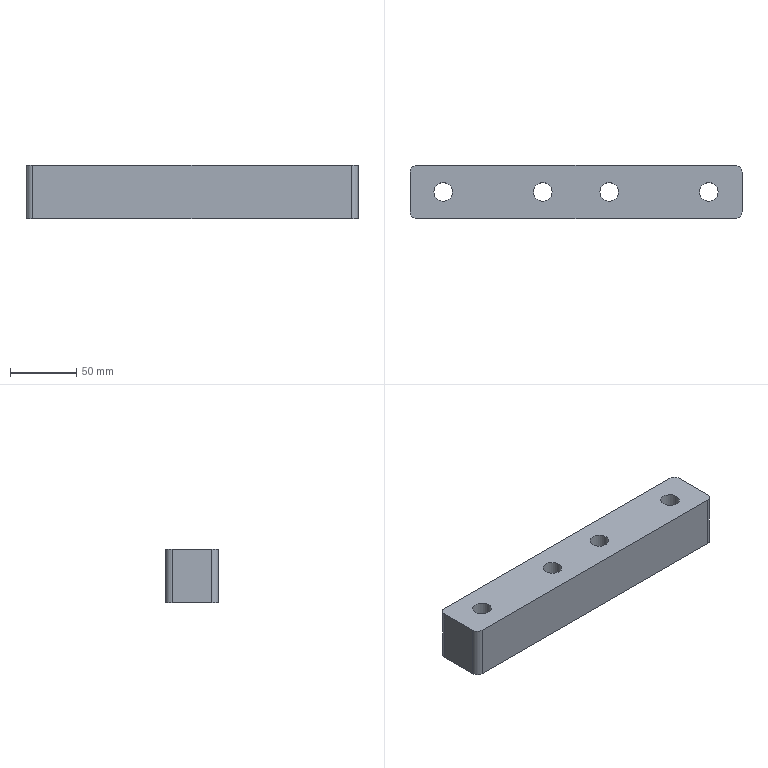Part | NX | features MAIN_BODY 2 | 1 solid | 14 faces | box 250 x 40 x 40 mm | volume 374512 mm3 | cylinder 8 | plane 6 | commonest cylinder face diameters 10 x4 14 x4
STEP:
#1=CARTESIAN_POINT('',(245.,825.,-195.));
#2=VERTEX_POINT('',#1);
#3=CARTESIAN_POINT('',(245.,795.,-195.));
#4=VERTEX_POINT('',#3);
#5=CARTESIAN_POINT('',(245.,830.,-195.));
#6=DIRECTION('',(0.,-1.,0.));
#7=VECTOR('',#6,1000.);
#8=LINE('',#5,#7);
#9=EDGE_CURVE('',#2,#4,#8,.T.);
#10=ORIENTED_EDGE('',*,*,#9,.F.);
#11=CARTESIAN_POINT('',(245.,825.,-235.));
#12=VERTEX_POINT('',#11);
#13=CARTESIAN_POINT('',(245.,825.,-235.));
#14=DIRECTION('',(0.,0.,1.));
#15=VECTOR('',#14,1000.);
#16=LINE('',#13,#15);
#17=EDGE_CURVE('',#2,#12,#16,.F.);
#18=ORIENTED_EDGE('',*,*,#17,.T.);
#19=CARTESIAN_POINT('',(245.,795.,-235.));
#20=VERTEX_POINT('',#19);
#21=CARTESIAN_POINT('',(245.,830.,-235.));
#22=DIRECTION('',(0.,-1.,0.));
#23=VECTOR('',#22,1000.);
#24=LINE('',#21,#23);
#25=EDGE_CURVE('',#12,#20,#24,.T.);
#26=ORIENTED_EDGE('',*,*,#25,.T.);
#27=CARTESIAN_POINT('',(245.,795.,-235.));
#28=DIRECTION('',(0.,0.,1.));
#29=VECTOR('',#28,1000.);
#30=LINE('',#27,#29);
#31=EDGE_CURVE('',#20,#4,#30,.T.);
#32=ORIENTED_EDGE('',*,*,#31,.T.);
#33=EDGE_LOOP('',(#10,#18,#26,#32));
#34=FACE_BOUND('',#33,.T.);
#35=CARTESIAN_POINT('',(245.,830.,-235.));
#36=DIRECTION('',(-1.,0.,0.));
#37=DIRECTION('',(0.,1.,0.));
#38=AXIS2_PLACEMENT_3D('',#35,#36,#37);
#39=PLANE('',#38);
#40=ADVANCED_FACE('',(#34),#39,.T.);
#41=CARTESIAN_POINT('',(250.,790.,-195.));
#42=VERTEX_POINT('',#41);
#43=CARTESIAN_POINT('',(490.,790.,-195.));
#44=VERTEX_POINT('',#43);
#45=CARTESIAN_POINT('',(245.,790.,-195.));
#46=DIRECTION('',(1.,0.,0.));
#47=VECTOR('',#46,1000.);
#48=LINE('',#45,#47);
#49=EDGE_CURVE('',#42,#44,#48,.T.);
#50=ORIENTED_EDGE('',*,*,#49,.F.);
#51=CARTESIAN_POINT('',(250.,790.,-235.));
#52=VERTEX_POINT('',#51);
#53=CARTESIAN_POINT('',(250.,790.,-235.));
#54=DIRECTION('',(0.,0.,1.));
#55=VECTOR('',#54,1000.);
#56=LINE('',#53,#55);
#57=EDGE_CURVE('',#42,#52,#56,.F.);
#58=ORIENTED_EDGE('',*,*,#57,.T.);
#59=CARTESIAN_POINT('',(490.,790.,-235.));
#60=VERTEX_POINT('',#59);
#61=CARTESIAN_POINT('',(245.,790.,-235.));
#62=DIRECTION('',(1.,0.,0.));
#63=VECTOR('',#62,1000.);
#64=LINE('',#61,#63);
#65=EDGE_CURVE('',#52,#60,#64,.T.);
#66=ORIENTED_EDGE('',*,*,#65,.T.);
#67=CARTESIAN_POINT('',(490.,790.,-235.));
#68=DIRECTION('',(0.,0.,1.));
#69=VECTOR('',#68,1000.);
#70=LINE('',#67,#69);
#71=EDGE_CURVE('',#60,#44,#70,.T.);
#72=ORIENTED_EDGE('',*,*,#71,.T.);
#73=EDGE_LOOP('',(#50,#58,#66,#72));
#74=FACE_BOUND('',#73,.T.);
#75=CARTESIAN_POINT('',(245.,790.,-235.));
#76=DIRECTION('',(0.,-1.,0.));
#77=DIRECTION('',(-1.,0.,0.));
#78=AXIS2_PLACEMENT_3D('',#75,#76,#77);
#79=PLANE('',#78);
#80=ADVANCED_FACE('',(#74),#79,.T.);
#81=CARTESIAN_POINT('',(490.,830.,-235.));
#82=VERTEX_POINT('',#81);
#83=CARTESIAN_POINT('',(250.,830.,-235.));
#84=VERTEX_POINT('',#83);
#85=CARTESIAN_POINT('',(370.,830.,-235.));
#86=DIRECTION('',(-1.,0.,0.));
#87=VECTOR('',#86,1000.);
#88=LINE('',#85,#87);
#89=EDGE_CURVE('',#82,#84,#88,.T.);
#90=ORIENTED_EDGE('',*,*,#89,.T.);
#91=CARTESIAN_POINT('',(250.,830.,-195.));
#92=VERTEX_POINT('',#91);
#93=CARTESIAN_POINT('',(250.,830.,-235.));
#94=DIRECTION('',(0.,0.,1.));
#95=VECTOR('',#94,1000.);
#96=LINE('',#93,#95);
#97=EDGE_CURVE('',#84,#92,#96,.T.);
#98=ORIENTED_EDGE('',*,*,#97,.T.);
#99=CARTESIAN_POINT('',(490.,830.,-195.));
#100=VERTEX_POINT('',#99);
#101=CARTESIAN_POINT('',(370.,830.,-195.));
#102=DIRECTION('',(-1.,0.,0.));
#103=VECTOR('',#102,1000.);
#104=LINE('',#101,#103);
#105=EDGE_CURVE('',#100,#92,#104,.T.);
#106=ORIENTED_EDGE('',*,*,#105,.F.);
#107=CARTESIAN_POINT('',(490.,830.,-235.));
#108=DIRECTION('',(0.,0.,1.));
#109=VECTOR('',#108,1000.);
#110=LINE('',#107,#109);
#111=EDGE_CURVE('',#100,#82,#110,.F.);
#112=ORIENTED_EDGE('',*,*,#111,.T.);
#113=EDGE_LOOP('',(#90,#98,#106,#112));
#114=FACE_BOUND('',#113,.T.);
#115=CARTESIAN_POINT('',(370.,830.,-235.));
#116=DIRECTION('',(0.,1.,0.));
#117=DIRECTION('',(0.,0.,-1.));
#118=AXIS2_PLACEMENT_3D('',#115,#116,#117);
#119=PLANE('',#118);
#120=ADVANCED_FACE('',(#114),#119,.T.);
#121=CARTESIAN_POINT('',(352.,810.,-235.));
#122=VERTEX_POINT('',#121);
#123=CARTESIAN_POINT('',(345.,810.,-235.));
#124=DIRECTION('',(0.,0.,1.));
#125=DIRECTION('',(1.,0.,0.));
#126=AXIS2_PLACEMENT_3D('',#123,#124,#125);
#127=CIRCLE('',#126,7.);
#128=EDGE_CURVE('',#122,#122,#127,.T.);
#129=ORIENTED_EDGE('',*,*,#128,.T.);
#130=EDGE_LOOP('',(#129));
#131=FACE_BOUND('',#130,.T.);
#132=CARTESIAN_POINT('',(277.,810.,-235.));
#133=VERTEX_POINT('',#132);
#134=CARTESIAN_POINT('',(270.,810.,-235.));
#135=DIRECTION('',(0.,0.,1.));
#136=DIRECTION('',(1.,0.,0.));
#137=AXIS2_PLACEMENT_3D('',#134,#135,#136);
#138=CIRCLE('',#137,7.);
#139=EDGE_CURVE('',#133,#133,#138,.T.);
#140=ORIENTED_EDGE('',*,*,#139,.T.);
#141=EDGE_LOOP('',(#140));
#142=FACE_BOUND('',#141,.T.);
#143=ORIENTED_EDGE('',*,*,#25,.F.);
#144=CARTESIAN_POINT('',(250.,825.,-235.));
#145=DIRECTION('',(0.,0.,1.));
#146=DIRECTION('',(1.,0.,0.));
#147=AXIS2_PLACEMENT_3D('',#144,#145,#146);
#148=CIRCLE('',#147,5.);
#149=EDGE_CURVE('',#12,#84,#148,.F.);
#150=ORIENTED_EDGE('',*,*,#149,.T.);
#151=ORIENTED_EDGE('',*,*,#89,.F.);
#152=CARTESIAN_POINT('',(495.,825.,-235.));
#153=VERTEX_POINT('',#152);
#154=CARTESIAN_POINT('',(490.,825.,-235.));
#155=DIRECTION('',(0.,0.,1.));
#156=DIRECTION('',(1.,0.,0.));
#157=AXIS2_PLACEMENT_3D('',#154,#155,#156);
#158=CIRCLE('',#157,5.);
#159=EDGE_CURVE('',#82,#153,#158,.F.);
#160=ORIENTED_EDGE('',*,*,#159,.T.);
#161=CARTESIAN_POINT('',(495.,795.,-235.));
#162=VERTEX_POINT('',#161);
#163=CARTESIAN_POINT('',(495.,830.,-235.));
#164=DIRECTION('',(0.,-1.,0.));
#165=VECTOR('',#164,1000.);
#166=LINE('',#163,#165);
#167=EDGE_CURVE('',#153,#162,#166,.T.);
#168=ORIENTED_EDGE('',*,*,#167,.T.);
#169=CARTESIAN_POINT('',(490.,795.,-235.));
#170=DIRECTION('',(0.,0.,1.));
#171=DIRECTION('',(1.,0.,0.));
#172=AXIS2_PLACEMENT_3D('',#169,#170,#171);
#173=CIRCLE('',#172,5.);
#174=EDGE_CURVE('',#162,#60,#173,.F.);
#175=ORIENTED_EDGE('',*,*,#174,.T.);
#176=ORIENTED_EDGE('',*,*,#65,.F.);
#177=CARTESIAN_POINT('',(250.,795.,-235.));
#178=DIRECTION('',(0.,0.,1.));
#179=DIRECTION('',(1.,0.,0.));
#180=AXIS2_PLACEMENT_3D('',#177,#178,#179);
#181=CIRCLE('',#180,5.);
#182=EDGE_CURVE('',#52,#20,#181,.F.);
#183=ORIENTED_EDGE('',*,*,#182,.T.);
#184=EDGE_LOOP('',(#143,#150,#151,#160,#168,#175,#176,#183));
#185=FACE_BOUND('',#184,.T.);
#186=CARTESIAN_POINT('',(388.,810.,-235.));
#187=VERTEX_POINT('',#186);
#188=CARTESIAN_POINT('',(395.,810.,-235.));
#189=DIRECTION('',(0.,0.,-1.));
#190=DIRECTION('',(-1.,0.,0.));
#191=AXIS2_PLACEMENT_3D('',#188,#189,#190);
#192=CIRCLE('',#191,7.);
#193=EDGE_CURVE('',#187,#187,#192,.T.);
#194=ORIENTED_EDGE('',*,*,#193,.F.);
#195=EDGE_LOOP('',(#194));
#196=FACE_BOUND('',#195,.T.);
#197=CARTESIAN_POINT('',(463.,810.,-235.));
#198=VERTEX_POINT('',#197);
#199=CARTESIAN_POINT('',(470.,810.,-235.));
#200=DIRECTION('',(0.,0.,-1.));
#201=DIRECTION('',(-1.,0.,0.));
#202=AXIS2_PLACEMENT_3D('',#199,#200,#201);
#203=CIRCLE('',#202,7.);
#204=EDGE_CURVE('',#198,#198,#203,.T.);
#205=ORIENTED_EDGE('',*,*,#204,.F.);
#206=EDGE_LOOP('',(#205));
#207=FACE_BOUND('',#206,.T.);
#208=CARTESIAN_POINT('',(245.,790.,-235.));
#209=DIRECTION('',(0.,0.,1.));
#210=DIRECTION('',(1.,0.,0.));
#211=AXIS2_PLACEMENT_3D('',#208,#209,#210);
#212=PLANE('',#211);
#213=ADVANCED_FACE('',(#131,#142,#185,#196,#207),#212,.F.);
#214=CARTESIAN_POINT('',(352.,810.,-195.));
#215=VERTEX_POINT('',#214);
#216=CARTESIAN_POINT('',(345.,810.,-195.));
#217=DIRECTION('',(0.,0.,1.));
#218=DIRECTION('',(1.,0.,0.));
#219=AXIS2_PLACEMENT_3D('',#216,#217,#218);
#220=CIRCLE('',#219,7.);
#221=EDGE_CURVE('',#215,#215,#220,.T.);
#222=ORIENTED_EDGE('',*,*,#221,.F.);
#223=EDGE_LOOP('',(#222));
#224=FACE_BOUND('',#223,.T.);
#225=CARTESIAN_POINT('',(277.,810.,-195.));
#226=VERTEX_POINT('',#225);
#227=CARTESIAN_POINT('',(270.,810.,-195.));
#228=DIRECTION('',(0.,0.,1.));
#229=DIRECTION('',(1.,0.,0.));
#230=AXIS2_PLACEMENT_3D('',#227,#228,#229);
#231=CIRCLE('',#230,7.);
#232=EDGE_CURVE('',#226,#226,#231,.T.);
#233=ORIENTED_EDGE('',*,*,#232,.F.);
#234=EDGE_LOOP('',(#233));
#235=FACE_BOUND('',#234,.T.);
#236=ORIENTED_EDGE('',*,*,#105,.T.);
#237=CARTESIAN_POINT('',(250.,825.,-195.));
#238=DIRECTION('',(0.,0.,1.));
#239=DIRECTION('',(1.,0.,0.));
#240=AXIS2_PLACEMENT_3D('',#237,#238,#239);
#241=CIRCLE('',#240,5.);
#242=EDGE_CURVE('',#92,#2,#241,.T.);
#243=ORIENTED_EDGE('',*,*,#242,.T.);
#244=ORIENTED_EDGE('',*,*,#9,.T.);
#245=CARTESIAN_POINT('',(250.,795.,-195.));
#246=DIRECTION('',(0.,0.,1.));
#247=DIRECTION('',(1.,0.,0.));
#248=AXIS2_PLACEMENT_3D('',#245,#246,#247);
#249=CIRCLE('',#248,5.);
#250=EDGE_CURVE('',#4,#42,#249,.T.);
#251=ORIENTED_EDGE('',*,*,#250,.T.);
#252=ORIENTED_EDGE('',*,*,#49,.T.);
#253=CARTESIAN_POINT('',(495.,795.,-195.));
#254=VERTEX_POINT('',#253);
#255=CARTESIAN_POINT('',(490.,795.,-195.));
#256=DIRECTION('',(0.,0.,1.));
#257=DIRECTION('',(1.,0.,0.));
#258=AXIS2_PLACEMENT_3D('',#255,#256,#257);
#259=CIRCLE('',#258,5.);
#260=EDGE_CURVE('',#44,#254,#259,.T.);
#261=ORIENTED_EDGE('',*,*,#260,.T.);
#262=CARTESIAN_POINT('',(495.,825.,-195.));
#263=VERTEX_POINT('',#262);
#264=CARTESIAN_POINT('',(495.,830.,-195.));
#265=DIRECTION('',(0.,-1.,0.));
#266=VECTOR('',#265,1000.);
#267=LINE('',#264,#266);
#268=EDGE_CURVE('',#263,#254,#267,.T.);
#269=ORIENTED_EDGE('',*,*,#268,.F.);
#270=CARTESIAN_POINT('',(490.,825.,-195.));
#271=DIRECTION('',(0.,0.,1.));
#272=DIRECTION('',(1.,0.,0.));
#273=AXIS2_PLACEMENT_3D('',#270,#271,#272);
#274=CIRCLE('',#273,5.);
#275=EDGE_CURVE('',#263,#100,#274,.T.);
#276=ORIENTED_EDGE('',*,*,#275,.T.);
#277=EDGE_LOOP('',(#236,#243,#244,#251,#252,#261,#269,#276));
#278=FACE_BOUND('',#277,.T.);
#279=CARTESIAN_POINT('',(388.,810.,-195.));
#280=VERTEX_POINT('',#279);
#281=CARTESIAN_POINT('',(395.,810.,-195.));
#282=DIRECTION('',(0.,0.,-1.));
#283=DIRECTION('',(-1.,0.,0.));
#284=AXIS2_PLACEMENT_3D('',#281,#282,#283);
#285=CIRCLE('',#284,7.);
#286=EDGE_CURVE('',#280,#280,#285,.T.);
#287=ORIENTED_EDGE('',*,*,#286,.T.);
#288=EDGE_LOOP('',(#287));
#289=FACE_BOUND('',#288,.T.);
#290=CARTESIAN_POINT('',(463.,810.,-195.));
#291=VERTEX_POINT('',#290);
#292=CARTESIAN_POINT('',(470.,810.,-195.));
#293=DIRECTION('',(0.,0.,-1.));
#294=DIRECTION('',(-1.,0.,0.));
#295=AXIS2_PLACEMENT_3D('',#292,#293,#294);
#296=CIRCLE('',#295,7.);
#297=EDGE_CURVE('',#291,#291,#296,.T.);
#298=ORIENTED_EDGE('',*,*,#297,.T.);
#299=EDGE_LOOP('',(#298));
#300=FACE_BOUND('',#299,.T.);
#301=CARTESIAN_POINT('',(245.,790.,-195.));
#302=DIRECTION('',(0.,0.,1.));
#303=DIRECTION('',(1.,0.,0.));
#304=AXIS2_PLACEMENT_3D('',#301,#302,#303);
#305=PLANE('',#304);
#306=ADVANCED_FACE('',(#224,#235,#278,#289,#300),#305,.T.);
#307=ORIENTED_EDGE('',*,*,#232,.T.);
#308=EDGE_LOOP('',(#307));
#309=FACE_BOUND('',#308,.T.);
#310=ORIENTED_EDGE('',*,*,#139,.F.);
#311=EDGE_LOOP('',(#310));
#312=FACE_BOUND('',#311,.T.);
#313=CARTESIAN_POINT('',(270.,810.,-235.));
#314=DIRECTION('',(0.,0.,1.));
#315=DIRECTION('',(1.,0.,0.));
#316=AXIS2_PLACEMENT_3D('',#313,#314,#315);
#317=CYLINDRICAL_SURFACE('',#316,7.);
#318=ADVANCED_FACE('',(#309,#312),#317,.F.);
#319=ORIENTED_EDGE('',*,*,#221,.T.);
#320=EDGE_LOOP('',(#319));
#321=FACE_BOUND('',#320,.T.);
#322=ORIENTED_EDGE('',*,*,#128,.F.);
#323=EDGE_LOOP('',(#322));
#324=FACE_BOUND('',#323,.T.);
#325=CARTESIAN_POINT('',(345.,810.,-235.));
#326=DIRECTION('',(0.,0.,1.));
#327=DIRECTION('',(1.,0.,0.));
#328=AXIS2_PLACEMENT_3D('',#325,#326,#327);
#329=CYLINDRICAL_SURFACE('',#328,7.);
#330=ADVANCED_FACE('',(#321,#324),#329,.F.);
#331=ORIENTED_EDGE('',*,*,#167,.F.);
#332=CARTESIAN_POINT('',(495.,825.,-235.));
#333=DIRECTION('',(0.,0.,1.));
#334=VECTOR('',#333,1000.);
#335=LINE('',#332,#334);
#336=EDGE_CURVE('',#153,#263,#335,.T.);
#337=ORIENTED_EDGE('',*,*,#336,.T.);
#338=ORIENTED_EDGE('',*,*,#268,.T.);
#339=CARTESIAN_POINT('',(495.,795.,-235.));
#340=DIRECTION('',(0.,0.,1.));
#341=VECTOR('',#340,1000.);
#342=LINE('',#339,#341);
#343=EDGE_CURVE('',#254,#162,#342,.F.);
#344=ORIENTED_EDGE('',*,*,#343,.T.);
#345=EDGE_LOOP('',(#331,#337,#338,#344));
#346=FACE_BOUND('',#345,.T.);
#347=CARTESIAN_POINT('',(495.,830.,-235.));
#348=DIRECTION('',(1.,0.,0.));
#349=DIRECTION('',(0.,1.,0.));
#350=AXIS2_PLACEMENT_3D('',#347,#348,#349);
#351=PLANE('',#350);
#352=ADVANCED_FACE('',(#346),#351,.T.);
#353=ORIENTED_EDGE('',*,*,#297,.F.);
#354=EDGE_LOOP('',(#353));
#355=FACE_BOUND('',#354,.T.);
#356=ORIENTED_EDGE('',*,*,#204,.T.);
#357=EDGE_LOOP('',(#356));
#358=FACE_BOUND('',#357,.T.);
#359=CARTESIAN_POINT('',(470.,810.,-235.));
#360=DIRECTION('',(0.,0.,1.));
#361=DIRECTION('',(-1.,0.,0.));
#362=AXIS2_PLACEMENT_3D('',#359,#360,#361);
#363=CYLINDRICAL_SURFACE('',#362,7.);
#364=ADVANCED_FACE('',(#355,#358),#363,.F.);
#365=ORIENTED_EDGE('',*,*,#286,.F.);
#366=EDGE_LOOP('',(#365));
#367=FACE_BOUND('',#366,.T.);
#368=ORIENTED_EDGE('',*,*,#193,.T.);
#369=EDGE_LOOP('',(#368));
#370=FACE_BOUND('',#369,.T.);
#371=CARTESIAN_POINT('',(395.,810.,-235.));
#372=DIRECTION('',(0.,0.,1.));
#373=DIRECTION('',(-1.,0.,0.));
#374=AXIS2_PLACEMENT_3D('',#371,#372,#373);
#375=CYLINDRICAL_SURFACE('',#374,7.);
#376=ADVANCED_FACE('',(#367,#370),#375,.F.);
#377=ORIENTED_EDGE('',*,*,#149,.F.);
#378=ORIENTED_EDGE('',*,*,#17,.F.);
#379=ORIENTED_EDGE('',*,*,#242,.F.);
#380=ORIENTED_EDGE('',*,*,#97,.F.);
#381=EDGE_LOOP('',(#377,#378,#379,#380));
#382=FACE_BOUND('',#381,.T.);
#383=CARTESIAN_POINT('',(250.,825.,-235.));
#384=DIRECTION('',(0.,0.,1.));
#385=DIRECTION('',(1.,0.,0.));
#386=AXIS2_PLACEMENT_3D('',#383,#384,#385);
#387=CYLINDRICAL_SURFACE('',#386,5.);
#388=ADVANCED_FACE('',(#382),#387,.T.);
#389=ORIENTED_EDGE('',*,*,#182,.F.);
#390=ORIENTED_EDGE('',*,*,#57,.F.);
#391=ORIENTED_EDGE('',*,*,#250,.F.);
#392=ORIENTED_EDGE('',*,*,#31,.F.);
#393=EDGE_LOOP('',(#389,#390,#391,#392));
#394=FACE_BOUND('',#393,.T.);
#395=CARTESIAN_POINT('',(250.,795.,-235.));
#396=DIRECTION('',(0.,0.,1.));
#397=DIRECTION('',(1.,0.,0.));
#398=AXIS2_PLACEMENT_3D('',#395,#396,#397);
#399=CYLINDRICAL_SURFACE('',#398,5.);
#400=ADVANCED_FACE('',(#394),#399,.T.);
#401=ORIENTED_EDGE('',*,*,#159,.F.);
#402=ORIENTED_EDGE('',*,*,#111,.F.);
#403=ORIENTED_EDGE('',*,*,#275,.F.);
#404=ORIENTED_EDGE('',*,*,#336,.F.);
#405=EDGE_LOOP('',(#401,#402,#403,#404));
#406=FACE_BOUND('',#405,.T.);
#407=CARTESIAN_POINT('',(490.,825.,-235.));
#408=DIRECTION('',(0.,0.,1.));
#409=DIRECTION('',(1.,0.,0.));
#410=AXIS2_PLACEMENT_3D('',#407,#408,#409);
#411=CYLINDRICAL_SURFACE('',#410,5.);
#412=ADVANCED_FACE('',(#406),#411,.T.);
#413=ORIENTED_EDGE('',*,*,#174,.F.);
#414=ORIENTED_EDGE('',*,*,#343,.F.);
#415=ORIENTED_EDGE('',*,*,#260,.F.);
#416=ORIENTED_EDGE('',*,*,#71,.F.);
#417=EDGE_LOOP('',(#413,#414,#415,#416));
#418=FACE_BOUND('',#417,.T.);
#419=CARTESIAN_POINT('',(490.,795.,-235.));
#420=DIRECTION('',(0.,0.,1.));
#421=DIRECTION('',(1.,0.,0.));
#422=AXIS2_PLACEMENT_3D('',#419,#420,#421);
#423=CYLINDRICAL_SURFACE('',#422,5.);
#424=ADVANCED_FACE('',(#418),#423,.T.);
#425=CLOSED_SHELL('',(#40,#80,#120,#213,#306,#318,#330,#352,#364,#376,#388,#400,#412,#424));
#426=MANIFOLD_SOLID_BREP('',#425);
#427=(LENGTH_UNIT()NAMED_UNIT(*)SI_UNIT(.MILLI.,.METRE.));
#428=UNCERTAINTY_MEASURE_WITH_UNIT(LENGTH_MEASURE(0.00001),#427,'','');
#429=(NAMED_UNIT(*)PLANE_ANGLE_UNIT()SI_UNIT($,.RADIAN.));
#430=(NAMED_UNIT(*)SI_UNIT($,.STERADIAN.)SOLID_ANGLE_UNIT());
#431=(GEOMETRIC_REPRESENTATION_CONTEXT(3)GLOBAL_UNCERTAINTY_ASSIGNED_CONTEXT((#428))GLOBAL_UNIT_ASSIGNED_CONTEXT((#427,#429,#430))REPRESENTATION_CONTEXT('',''));
#432=ADVANCED_BREP_SHAPE_REPRESENTATION('',(#426),#431);